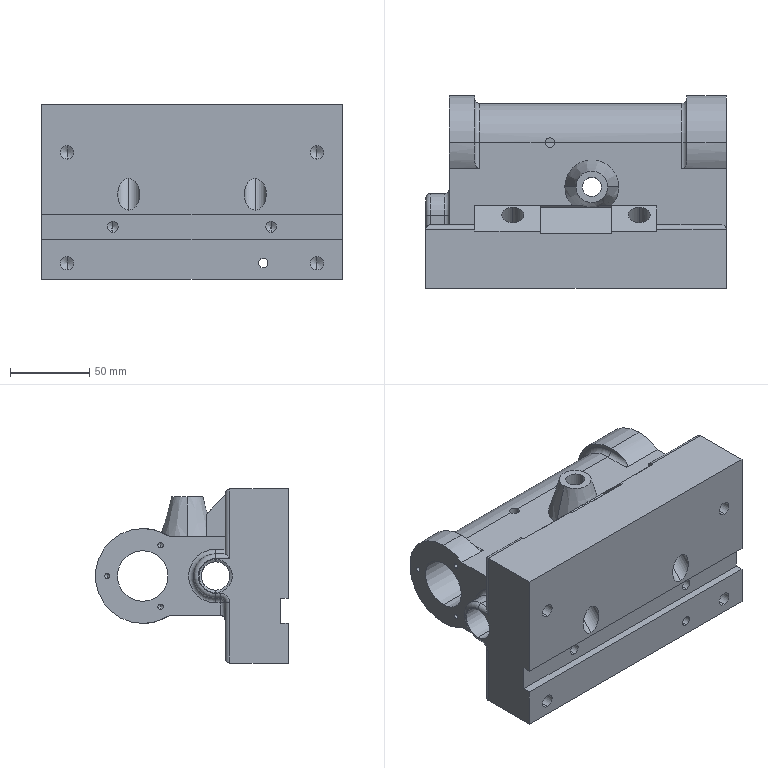Part | SolidWorks | features ICE 19, HoleWzd 6, Fillet 3, Extrusion 1, Revolution 1 | 1 solid | 155 faces | box 190 x 122 x 110 mm | volume 1237732 mm3 | cylinder 79 | plane 37 | cone 32 | torus 6 | sphere 1 | commonest cylinder face diameters 6 x23 4.2 x8 8.5 x8 3.3 x6 60 x6 6.8 x4